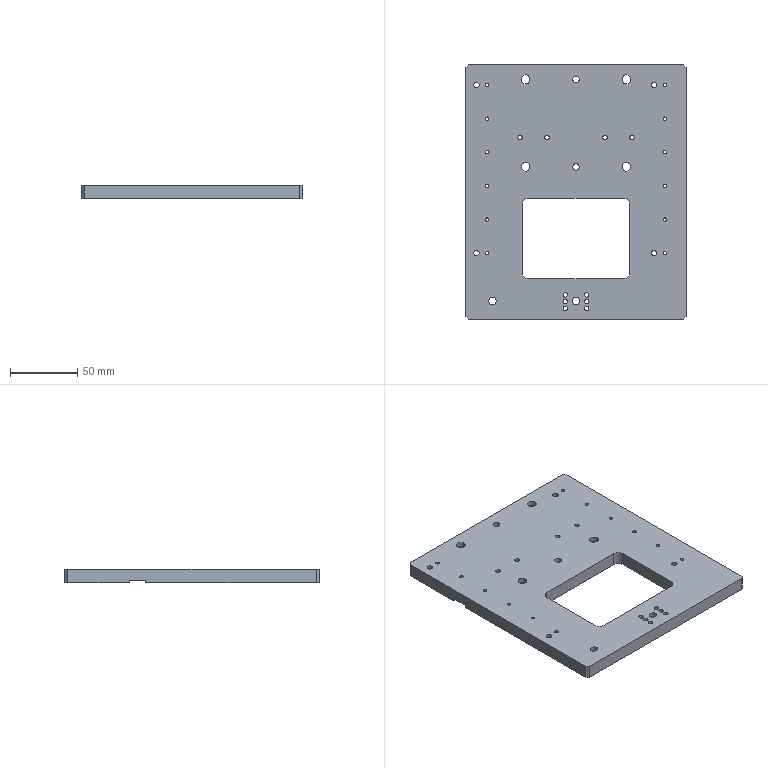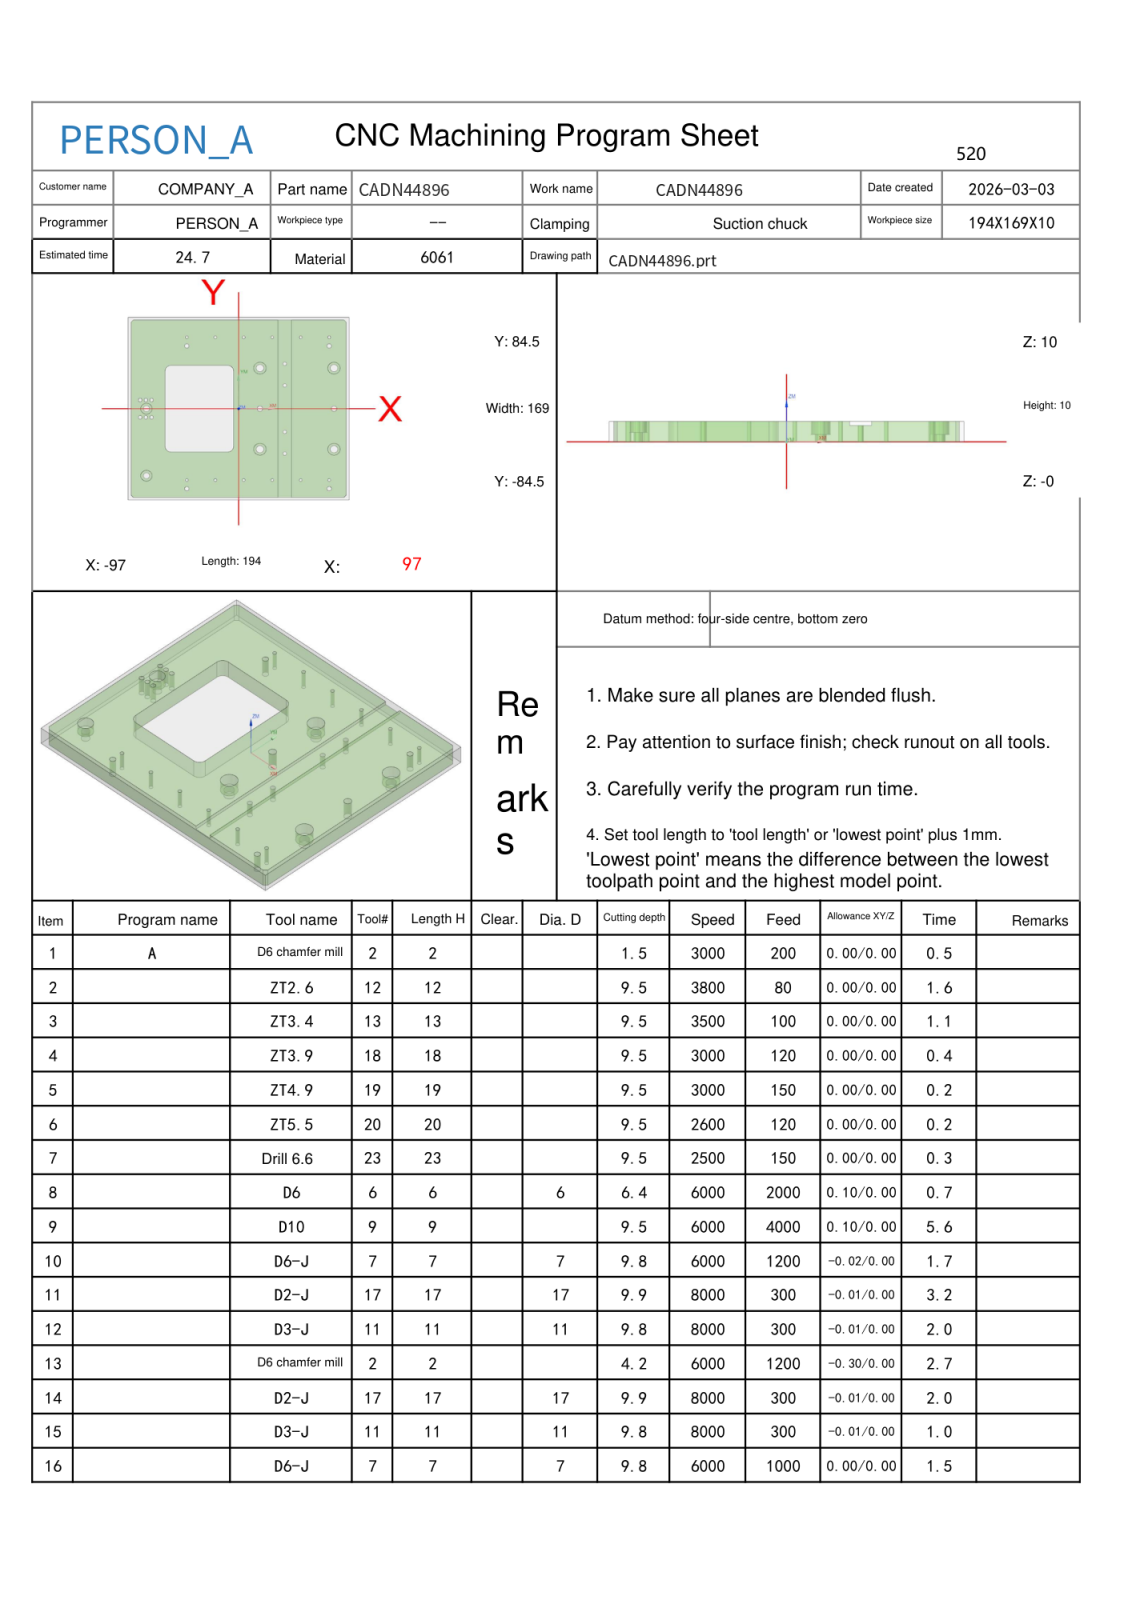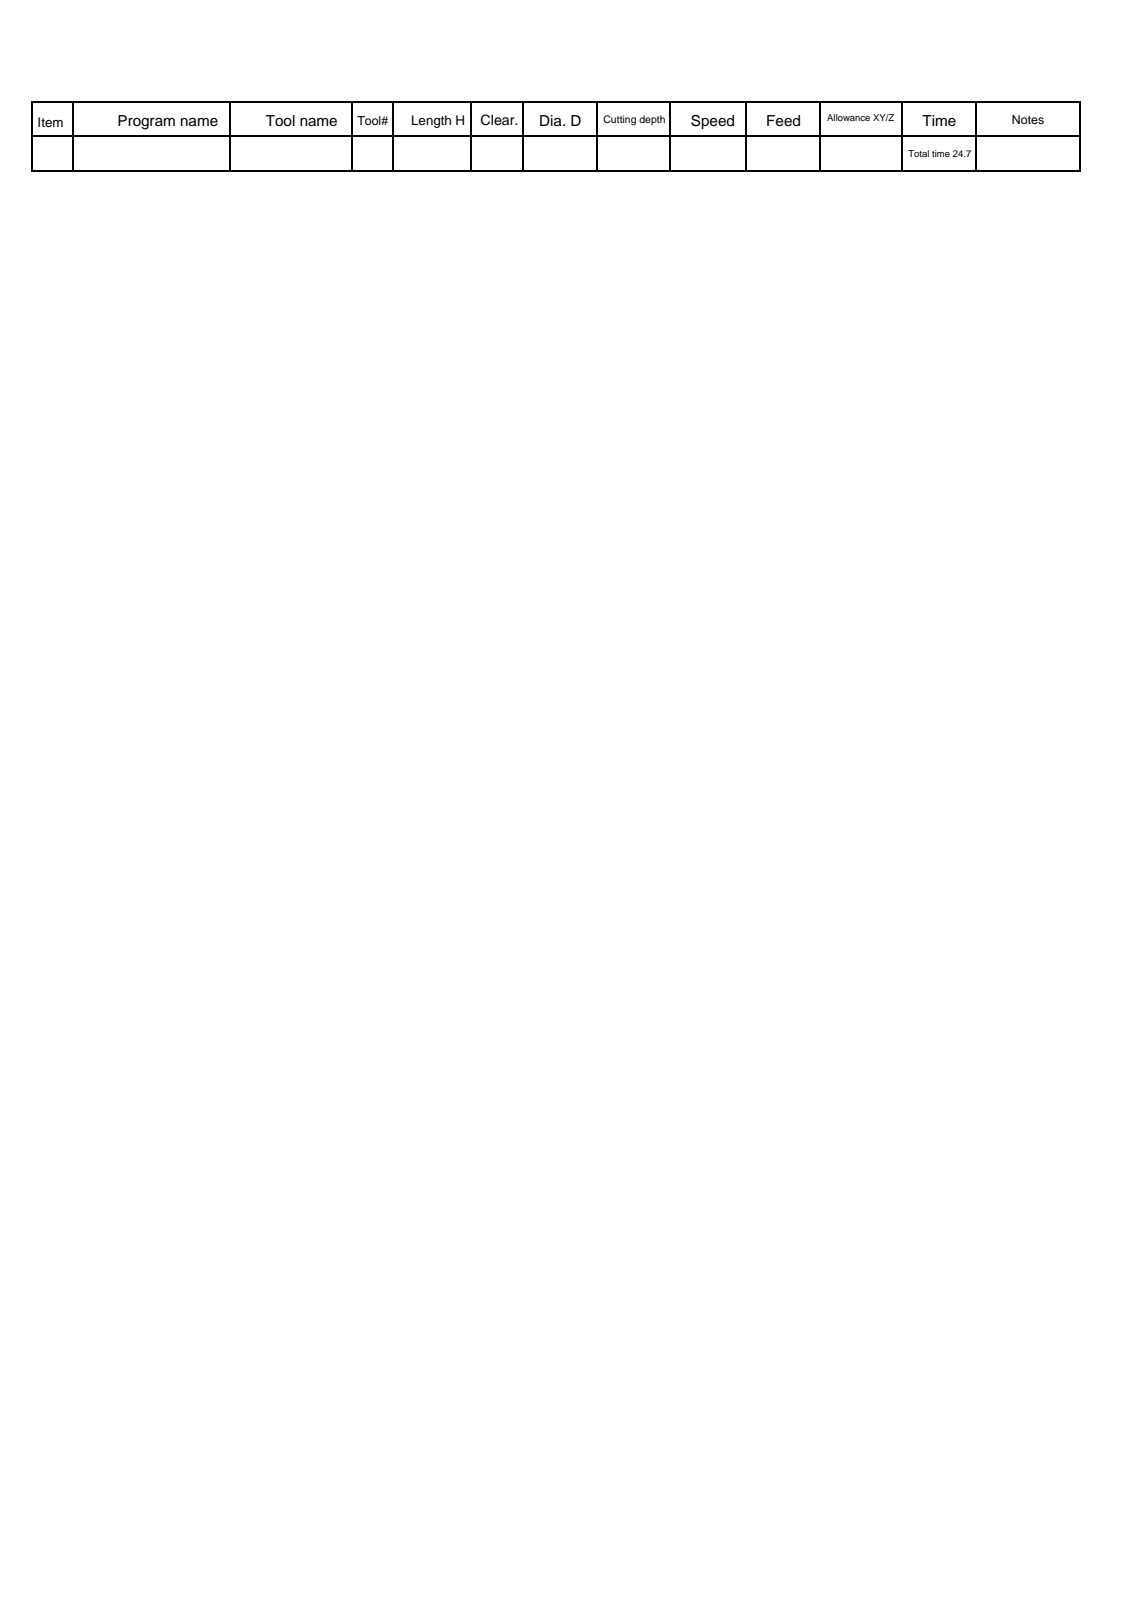NC program | NX | posted by the shop | part box 164 x 189 x 10 mm
Lines 1 to 1038 of 4061:
%
O0001
(Machine time: 27.66 MIN)
(===Total Tool:12===)
(T2=D6 chamfer mill   D=6.   R=0.   D-  H02 Z=5.8   )
(T12=ZT2.6  D=2.6  DR_a=118 D-  H12 Z=0.5   )
(T13=ZT3.4  D=3.4  DR_a=118 D-  H13 Z=0.5   )
(T18=ZT3.9  D=3.9  DR_a=120 D-  H18 Z=0.5   )
(T19=ZT4.9  D=4.9  DR_a=120 D-  H19 Z=0.5   )
(T20=ZT5.5  D=5.5  DR_a=118 D-  H20 Z=0.5   )
(T23=Drill 6.6  D=6.6  DR_a=120 D-  H23 Z=0.5   )
(T6=D6      D=6.   R=0.   D6  H06 Z=3.6   )
(T9=D10     D=10.  R=0.   D-  H09 Z=0.5   )
(T7=D6-J    D=6.   R=0.   D7  H07 Z=0.2   )
(T17=D2-J   D=2.   R=0.   D17 H17 Z=0.15  )
(T11=D3-J   D=3.   R=0.   D11 H11 Z=0.15  )
G80 G90 G17 G49 G40
G91 G28 Z0
M01
N1 T02 M06
(D6 chamfer mill  D=6. R=0. H=02 ce=0.00 di=0.00)
(MAX_Z=40. MIN_Z=8.5 Time=0.49M)
G00 G90 G54 X83.7 Y0.0 M03 S3000
G43 H02 Z40.
M08
G98 G82 X83.7 Y0.0 Z8.5 R11. F200.
X18.7
G80
G00 Z40.
G00 G90 X79.5 Y-66. M03 S3000
Z40.
G98 G81 X79.5 Y-66. Z9. R11. F200.
X54.5
X29.5
X4.5
X-20.5
X-45.5
Y66.
X-20.5
X4.5
X29.5
X54.5
X79.5
G80
G00 Z40.
G00 G90 X83.7 Y37.5 M03 S3000
Z40.
G98 G81 X83.7 Y37.5 Z8.5 R11. F200.
X79.5 Y58.
X40.5 Y41.5
X18.7 Y37.5
X40.5 Y21.5
Y-21.5
X83.7 Y-37.5
X79.5 Y-74.
X40.5 Y-41.5
X18.7 Y-37.5
X-45.5 Y-74.
X-81. Y-62.
X-86.5 Y-8.
X-81.5
X-76.5
X-81. Y0.0
X-86.5 Y8.
X-81.5
X-76.5
X-45.5 Y58.
G80
G00 Z40.
G91 G28 Z0.0
M05
M09
G91 G28 Z0.0
M01
N2 T12 M06
(ZT2.6 D=2.6 DR_a=118 H=12)
(MAX_Z=40. MIN_Z=0.5 Time=1.62M)
G00 G90 G54 X79.5 Y-66. M03 S3800
G43 H12 Z40.
M08
G98 G83 X79.5 Y-66. Z.5 R11. F80. Q1.5
X54.5
X29.5
X4.5
X-20.5
X-45.5
Y66.
X-20.5
X4.5
X29.5
X54.5
X79.5
G80
G00 Z40.
G91 G28 Z0.0
M05
M09
G91 G28 Z0.0
M01
N3 T13 M06
(ZT3.4 D=3.4 DR_a=118 H=13)
(MAX_Z=40. MIN_Z=0.5 Time=1.08M)
G00 G90 G54 X-76.5 Y-8. M03 S3500
G43 H13 Z40.
M08
G98 G83 X-76.5 Y-8. Z.5 R11. F100. Q1.5
X-81.5
X-86.5
Y8.
X-81.5
X-76.5
X40.5 Y41.5
Y21.5
Y-21.5
Y-41.5
G80
G00 Z40.
G91 G28 Z0.0
M05
M09
G91 G28 Z0.0
M01
N4 T18 M06
(ZT3.9 D=3.9 DR_a=120 H=18)
(MAX_Z=40. MIN_Z=0.5 Time=0.39M)
G00 G90 G54 X-45.5 Y-74. M03 S3000
G43 H18 Z40.
M08
G98 G83 X-45.5 Y-74. Z.5 R11. F120. Q2.
X79.5
Y58.
X-45.5
G80
G00 Z40.
G91 G28 Z0.0
M05
M09
G91 G28 Z0.0
M01
N5 T19 M06
(ZT4.9 D=4.9 DR_a=120 H=19)
(MAX_Z=40. MIN_Z=0.5 Time=0.16M)
G00 G90 G54 X83.7 Y0.0 M03 S3000
G43 H19 Z40.
M08
G98 G83 X83.7 Y0.0 Z.5 R11. F150. Q3.
X18.7
G80
G00 Z40.
G91 G28 Z0.0
M05
M09
G91 G28 Z0.0
M01
N6 T20 M06
(ZT5.5 D=5.5 DR_a=118 H=20)
(MAX_Z=40. MIN_Z=0.5 Time=0.19M)
G00 G90 G54 X-81. Y0.0 M03 S2600
G43 H20 Z40.
M08
G98 G83 X-81. Y0.0 Z.5 R11. F120. Q3.
Y-62.
G80
G00 Z40.
G91 G28 Z0.0
M05
M09
G91 G28 Z0.0
M01
N7 T23 M06
(Drill 6.6 D=6.6 DR_a=120 H=23)
(MAX_Z=40. MIN_Z=0.5 Time=0.31M)
G00 G90 G54 X83.7 Y37.5 M03 S2500
G43 H23 Z40.
M08
G98 G83 X83.7 Y37.5 Z.5 R11. F150. Q3.
X18.7
Y-37.5
X83.7
G80
G00 Z40.
G91 G28 Z0.0
M05
M09
G91 G28 Z0.0
M01
N8 T06 M06
(D6  D=6. R=0. H=06 ce=0.10 di=0.00)
(D.N=06 MAX_Z=40. MIN_Z=3.6 Time=0.72M)
G00 G90 G54 X-81. Y0.0 M03 S6000
G43 H06 Z40.
M08
Z10.3
G41 D06
G01 X-80.9 Y-.007 F2000.
G03 X-80.044 Y.944 I-.1 J.951
X-81. Y1.9 I-.956 J0.0
X-81. Y1.9 Z9.95 I0.0 J-1.9
X-81. Y1.9 Z9.6 I0.0 J-1.9
X-81. Y1.9 Z9.25 I0.0 J-1.9
X-81. Y1.9 Z8.9 I0.0 J-1.9
X-81. Y1.9 Z8.55 I0.0 J-1.9
X-81. Y1.9 Z8.2 I0.0 J-1.9
X-81. Y1.9 Z7.85 I0.0 J-1.9
X-81. Y1.9 Z7.5 I0.0 J-1.9
X-81. Y1.9 Z7.15 I0.0 J-1.9
X-81. Y1.9 Z6.8 I0.0 J-1.9
X-81. Y1.9 Z6.45 I0.0 J-1.9
X-81. Y1.9 Z6.1 I0.0 J-1.9
X-81. Y1.9 Z5.75 I0.0 J-1.9
X-81. Y1.9 Z5.4 I0.0 J-1.9
X-81. Y1.9 Z5.05 I0.0 J-1.9
X-81. Y1.9 Z4.7 I0.0 J-1.9
X-82.852 Y-.423 Z4.6 I0.0 J-1.9
X-81. Y-1.9 I1.852 J.423
X-79.1 Y0.0 I0.0 J1.9
X-81. Y1.9 I-1.9 J0.0
X-82.9 Y0.0 I0.0 J-1.9
X-82.852 Y-.423 I1.9 J0.0
X-81.92 Y-1.166 I.932 J.213
X-80.964 Y-.21 I0.0 J.956
G01 X-80.971 Y-.096
G40 X-81. Y0.0
G00 Z40.
Y-62.
Z10.3
G41 D06
G01 X-80.9 Y-62.007
G03 X-80.044 Y-61.056 I-.1 J.951
X-81. Y-60.1 I-.956 J0.0
X-81. Y-60.1 Z9.95 I0.0 J-1.9
X-81. Y-60.1 Z9.6 I0.0 J-1.9
X-81. Y-60.1 Z9.25 I0.0 J-1.9
X-81. Y-60.1 Z8.9 I0.0 J-1.9
X-81. Y-60.1 Z8.55 I0.0 J-1.9
X-81. Y-60.1 Z8.2 I0.0 J-1.9
X-81. Y-60.1 Z7.85 I0.0 J-1.9
X-81. Y-60.1 Z7.5 I0.0 J-1.9
X-81. Y-60.1 Z7.15 I0.0 J-1.9
X-81. Y-60.1 Z6.8 I0.0 J-1.9
X-81. Y-60.1 Z6.45 I0.0 J-1.9
X-81. Y-60.1 Z6.1 I0.0 J-1.9
X-81. Y-60.1 Z5.75 I0.0 J-1.9
X-81. Y-60.1 Z5.4 I0.0 J-1.9
X-81. Y-60.1 Z5.05 I0.0 J-1.9
X-81. Y-60.1 Z4.7 I0.0 J-1.9
X-82.852 Y-62.423 Z4.6 I0.0 J-1.9
X-81. Y-63.9 I1.852 J.423
X-79.1 Y-62. I0.0 J1.9
X-81. Y-60.1 I-1.9 J0.0
X-82.9 Y-62. I0.0 J-1.9
X-82.852 Y-62.423 I1.9 J0.0
X-81.92 Y-63.166 I.932 J.213
X-80.964 Y-62.21 I0.0 J.956
G01 X-80.971 Y-62.096
G40 X-81. Y-62.
G00 Z40.
G00 G90 X18.7 Y-37.5 M03 S6000
Z40.
Z10.3
G03 X19.9 Y-36.3 I0.0 J1.2 F2000.
X18.7 Y-35.1 I-1.2 J0.0
X18.7 Y-35.1 Z9.8 I0.0 J-2.4
X18.7 Y-35.1 Z9.3 I0.0 J-2.4
X18.7 Y-35.1 Z8.8 I0.0 J-2.4
X18.7 Y-35.1 Z8.3 I0.0 J-2.4
X18.7 Y-35.1 Z7.8 I0.0 J-2.4
X18.7 Y-35.1 Z7.3 I0.0 J-2.4
X18.7 Y-35.1 Z6.8 I0.0 J-2.4
X18.7 Y-35.1 Z6.3 I0.0 J-2.4
X18.7 Y-35.1 Z5.8 I0.0 J-2.4
X18.7 Y-35.1 Z5.3 I0.0 J-2.4
X18.7 Y-35.1 Z4.8 I0.0 J-2.4
X18.7 Y-35.1 Z4.3 I0.0 J-2.4
X18.7 Y-35.1 Z3.8 I0.0 J-2.4
X17.289 Y-39.442 Z3.6 I0.0 J-2.4
X18.7 Y-39.9 I1.411 J1.942
X21.1 Y-37.5 I0.0 J2.4
X18.7 Y-35.1 I-2.4 J0.0
X16.3 Y-37.5 I0.0 J-2.4
X17.289 Y-39.442 I2.4 J0.0
X17.995 Y-39.671 I.705 J.971
X19.195 Y-38.471 I0.0 J1.2
X18.7 Y-37.5 I-1.2 J0.0
G00 Z40.
X83.7
Z10.3
G03 X84.9 Y-36.3 I0.0 J1.2
X83.7 Y-35.1 I-1.2 J0.0
X83.7 Y-35.1 Z9.8 I0.0 J-2.4
X83.7 Y-35.1 Z9.3 I0.0 J-2.4
X83.7 Y-35.1 Z8.8 I0.0 J-2.4
X83.7 Y-35.1 Z8.3 I0.0 J-2.4
X83.7 Y-35.1 Z7.8 I0.0 J-2.4
X83.7 Y-35.1 Z7.3 I0.0 J-2.4
X83.7 Y-35.1 Z6.8 I0.0 J-2.4
X83.7 Y-35.1 Z6.3 I0.0 J-2.4
X83.7 Y-35.1 Z5.8 I0.0 J-2.4
X83.7 Y-35.1 Z5.3 I0.0 J-2.4
X83.7 Y-35.1 Z4.8 I0.0 J-2.4
X83.7 Y-35.1 Z4.3 I0.0 J-2.4
X83.7 Y-35.1 Z3.8 I0.0 J-2.4
X82.289 Y-39.442 Z3.6 I0.0 J-2.4
X83.7 Y-39.9 I1.411 J1.942
X86.1 Y-37.5 I0.0 J2.4
X83.7 Y-35.1 I-2.4 J0.0
X81.3 Y-37.5 I0.0 J-2.4
X82.289 Y-39.442 I2.4 J0.0
X82.995 Y-39.671 I.705 J.971
X84.195 Y-38.471 I0.0 J1.2
X83.7 Y-37.5 I-1.2 J0.0
G00 Z40.
Y37.5
Z10.3
G03 X84.9 Y38.7 I0.0 J1.2
X83.7 Y39.9 I-1.2 J0.0
X83.7 Y39.9 Z9.8 I0.0 J-2.4
X83.7 Y39.9 Z9.3 I0.0 J-2.4
X83.7 Y39.9 Z8.8 I0.0 J-2.4
X83.7 Y39.9 Z8.3 I0.0 J-2.4
X83.7 Y39.9 Z7.8 I0.0 J-2.4
X83.7 Y39.9 Z7.3 I0.0 J-2.4
X83.7 Y39.9 Z6.8 I0.0 J-2.4
X83.7 Y39.9 Z6.3 I0.0 J-2.4
X83.7 Y39.9 Z5.8 I0.0 J-2.4
X83.7 Y39.9 Z5.3 I0.0 J-2.4
X83.7 Y39.9 Z4.8 I0.0 J-2.4
X83.7 Y39.9 Z4.3 I0.0 J-2.4
X83.7 Y39.9 Z3.8 I0.0 J-2.4
X82.289 Y35.558 Z3.6 I0.0 J-2.4
X83.7 Y35.1 I1.411 J1.942
X86.1 Y37.5 I0.0 J2.4
X83.7 Y39.9 I-2.4 J0.0
X81.3 Y37.5 I0.0 J-2.4
X82.289 Y35.558 I2.4 J0.0
X82.995 Y35.329 I.705 J.971
X84.195 Y36.529 I0.0 J1.2
X83.7 Y37.5 I-1.2 J0.0
G00 Z40.
X18.7
Z10.3
G03 X19.9 Y38.7 I0.0 J1.2
X18.7 Y39.9 I-1.2 J0.0
X18.7 Y39.9 Z9.8 I0.0 J-2.4
X18.7 Y39.9 Z9.3 I0.0 J-2.4
X18.7 Y39.9 Z8.8 I0.0 J-2.4
X18.7 Y39.9 Z8.3 I0.0 J-2.4
X18.7 Y39.9 Z7.8 I0.0 J-2.4
X18.7 Y39.9 Z7.3 I0.0 J-2.4
X18.7 Y39.9 Z6.8 I0.0 J-2.4
X18.7 Y39.9 Z6.3 I0.0 J-2.4
X18.7 Y39.9 Z5.8 I0.0 J-2.4
X18.7 Y39.9 Z5.3 I0.0 J-2.4
X18.7 Y39.9 Z4.8 I0.0 J-2.4
X18.7 Y39.9 Z4.3 I0.0 J-2.4
X18.7 Y39.9 Z3.8 I0.0 J-2.4
X17.289 Y35.558 Z3.6 I0.0 J-2.4
X18.7 Y35.1 I1.411 J1.942
X21.1 Y37.5 I0.0 J2.4
X18.7 Y39.9 I-2.4 J0.0
X16.3 Y37.5 I0.0 J-2.4
X17.289 Y35.558 I2.4 J0.0
X17.995 Y35.329 I.705 J.971
X19.195 Y36.529 I0.0 J1.2
X18.7 Y37.5 I-1.2 J0.0
G00 Z40.
G91 G28 Z0.0
M05
M09
G91 G28 Z0.0
M01
N9 T09 M06
(D10  D=10. R=0. H=09 ce=0.10 di=0.10)
(MAX_Z=40. MIN_Z=0.5 Time=5.57M)
G00 G90 G54 X41.4 Y46.666 M03 S6000
G43 H09 Z40.
M08
Z10.5
G01 Y83. Z9.549 F3500.
X40.5 Z9.525
X39.6
Y-83.
X41.4
Y83.
X40.5
X40.
Z10.025
G00 Z10.5
X41.4 Y46.666
Z10.025
G01 Y83. Z9.074
X40.5 Z9.05
X39.6
Y-83.
X41.4
Y83.
X40.5
X40.
Z9.55
G00 Z10.025
X41.4 Y46.666
Z9.55
G01 Y83. Z8.599
X40.5 Z8.575
X39.6
Y-83.
X41.4
Y83.
X40.5
X40.
Z9.075
G00 Z9.55
X41.4 Y46.666
Z9.075
G01 Y83. Z8.124
X40.5 Z8.1
X39.6
Y-83.
X41.4
Y83.
X40.5
X40.
Z8.6
G00 Z40.
G00 G90 X-59.4 Y0.0 M03 S6000
Z40.
Z10.5
G01 Y-34.9 Z10.427 F4000.
X-9.6 Z10.323
Y34.9 Z10.177
X-59.4 Z10.073
Y-34.9 Z9.927
X-9.6 Z9.823
Y34.9 Z9.677
X-59.4 Z9.573
Y-34.9 Z9.427
X-9.6 Z9.323
Y34.9 Z9.177
X-59.4 Z9.073
Y-34.9 Z8.927
X-9.6 Z8.823
Y34.9 Z8.677
X-59.4 Z8.573
Y-34.9 Z8.427
X-9.6 Z8.323
Y34.9 Z8.177
X-59.4 Z8.073
Y-34.9 Z7.927
X-9.6 Z7.823
Y34.9 Z7.677
X-59.4 Z7.573
Y-34.9 Z7.427
X-9.6 Z7.323
Y34.9 Z7.177
X-59.4 Z7.073
Y-34.9 Z6.927
X-9.6 Z6.823
Y34.9 Z6.677
X-59.4 Z6.573
Y-34.9 Z6.427
X-9.6 Z6.323
Y34.9 Z6.177
X-59.4 Z6.073
Y-34.9 Z5.927
X-9.6 Z5.823
Y34.9 Z5.677
X-59.4 Z5.573
Y-34.9 Z5.427
X-9.6 Z5.323
Y34.9 Z5.177
X-59.4 Z5.073
Y-34.9 Z4.927
X-9.6 Z4.823
Y34.9 Z4.677
X-59.4 Z4.573
Y-34.9 Z4.427
X-9.6 Z4.323
Y34.9 Z4.177
X-59.4 Z4.073
Y-34.9 Z3.927
X-9.6 Z3.823
Y34.9 Z3.677
X-59.4 Z3.573
Y-34.9 Z3.427
X-9.6 Z3.323
Y34.9 Z3.177
X-59.4 Z3.073
Y-34.9 Z2.927
X-9.6 Z2.823
Y34.9 Z2.677
X-59.4 Z2.573
Y-34.9 Z2.427
X-9.6 Z2.323
Y34.9 Z2.177
X-59.4 Z2.073
Y-34.9 Z1.927
X-9.6 Z1.823
Y34.9 Z1.677
X-59.4 Z1.573
Y-34.9 Z1.427
X-9.6 Z1.323
Y34.9 Z1.177
X-59.4 Z1.073
Y-34.9 Z.927
X-9.6 Z.823
Y34.9 Z.677
X-59.4 Z.573
Y0.0 Z.5
Y-34.9
X-9.6
Y34.9
X-59.4
Y0.0
Y-.5
Z1.5
G00 Z40.
G00 G90 X0.0 Y-87.1 M03 S6000
Z40.
Z10.5
G01 X-92.5 Z10.437 F4000.
G02 X-96.106 Y-85.606 Z10.434 I0.0 J5.1
G01 X-98.106 Y-83.606 Z10.432
G02 X-99.6 Y-80. Z10.43 I3.606 J3.606
G01 Y80. Z10.32
G02 X-98.106 Y83.606 Z10.318 I5.1 J0.0
G01 X-96.106 Y85.606 Z10.316
G02 X-92.5 Y87.1 Z10.313 I3.606 J-3.606
G01 X92.5 Z10.187
G02 X96.106 Y85.606 Z10.184 I0.0 J-5.1
G01 X98.106 Y83.606 Z10.182
G02 X99.6 Y80. Z10.18 I-3.606 J-3.606
G01 Y-80. Z10.07
G02 X98.106 Y-83.606 Z10.068 I-5.1 J0.0
G01 X96.106 Y-85.606 Z10.066
G02 X92.5 Y-87.1 Z10.063 I-3.606 J3.606
G01 X-92.5 Z9.937
G02 X-96.106 Y-85.606 Z9.934 I0.0 J5.1
G01 X-98.106 Y-83.606 Z9.932
G02 X-99.6 Y-80. Z9.93 I3.606 J3.606
G01 Y80. Z9.82
G02 X-98.106 Y83.606 Z9.818 I5.1 J0.0
G01 X-96.106 Y85.606 Z9.816
G02 X-92.5 Y87.1 Z9.813 I3.606 J-3.606
G01 X92.5 Z9.687
G02 X96.106 Y85.606 Z9.684 I0.0 J-5.1
G01 X98.106 Y83.606 Z9.682
G02 X99.6 Y80. Z9.68 I-3.606 J-3.606
G01 Y-80. Z9.57
G02 X98.106 Y-83.606 Z9.568 I-5.1 J0.0
G01 X96.106 Y-85.606 Z9.566
G02 X92.5 Y-87.1 Z9.563 I-3.606 J3.606
G01 X-92.5 Z9.437
G02 X-96.106 Y-85.606 Z9.434 I0.0 J5.1
G01 X-98.106 Y-83.606 Z9.432
G02 X-99.6 Y-80. Z9.43 I3.606 J3.606
G01 Y80. Z9.32
G02 X-98.106 Y83.606 Z9.318 I5.1 J0.0
G01 X-96.106 Y85.606 Z9.316
G02 X-92.5 Y87.1 Z9.313 I3.606 J-3.606
G01 X92.5 Z9.187
G02 X96.106 Y85.606 Z9.184 I0.0 J-5.1
G01 X98.106 Y83.606 Z9.182
G02 X99.6 Y80. Z9.18 I-3.606 J-3.606
G01 Y-80. Z9.07
G02 X98.106 Y-83.606 Z9.068 I-5.1 J0.0
G01 X96.106 Y-85.606 Z9.066
G02 X92.5 Y-87.1 Z9.063 I-3.606 J3.606
G01 X-92.5 Z8.937
G02 X-96.106 Y-85.606 Z8.934 I0.0 J5.1
G01 X-98.106 Y-83.606 Z8.932
G02 X-99.6 Y-80. Z8.93 I3.606 J3.606
G01 Y80. Z8.82
G02 X-98.106 Y83.606 Z8.818 I5.1 J0.0
G01 X-96.106 Y85.606 Z8.816
G02 X-92.5 Y87.1 Z8.813 I3.606 J-3.606
G01 X92.5 Z8.687
G02 X96.106 Y85.606 Z8.684 I0.0 J-5.1
G01 X98.106 Y83.606 Z8.682
G02 X99.6 Y80. Z8.68 I-3.606 J-3.606
G01 Y-80. Z8.57
G02 X98.106 Y-83.606 Z8.568 I-5.1 J0.0
G01 X96.106 Y-85.606 Z8.566
G02 X92.5 Y-87.1 Z8.563 I-3.606 J3.606
G01 X-92.5 Z8.437
G02 X-96.106 Y-85.606 Z8.434 I0.0 J5.1
G01 X-98.106 Y-83.606 Z8.432
G02 X-99.6 Y-80. Z8.43 I3.606 J3.606
G01 Y80. Z8.32
G02 X-98.106 Y83.606 Z8.318 I5.1 J0.0
G01 X-96.106 Y85.606 Z8.316
G02 X-92.5 Y87.1 Z8.313 I3.606 J-3.606
G01 X92.5 Z8.187
G02 X96.106 Y85.606 Z8.184 I0.0 J-5.1
G01 X98.106 Y83.606 Z8.182
G02 X99.6 Y80. Z8.18 I-3.606 J-3.606
G01 Y-80. Z8.07
G02 X98.106 Y-83.606 Z8.068 I-5.1 J0.0
G01 X96.106 Y-85.606 Z8.066
G02 X92.5 Y-87.1 Z8.063 I-3.606 J3.606
G01 X-92.5 Z7.937
G02 X-96.106 Y-85.606 Z7.934 I0.0 J5.1
G01 X-98.106 Y-83.606 Z7.932
G02 X-99.6 Y-80. Z7.93 I3.606 J3.606
G01 Y80. Z7.82
G02 X-98.106 Y83.606 Z7.818 I5.1 J0.0
G01 X-96.106 Y85.606 Z7.816
G02 X-92.5 Y87.1 Z7.813 I3.606 J-3.606
G01 X92.5 Z7.687
G02 X96.106 Y85.606 Z7.684 I0.0 J-5.1
G01 X98.106 Y83.606 Z7.682
G02 X99.6 Y80. Z7.68 I-3.606 J-3.606
G01 Y-80. Z7.57
G02 X98.106 Y-83.606 Z7.568 I-5.1 J0.0
G01 X96.106 Y-85.606 Z7.566
G02 X92.5 Y-87.1 Z7.563 I-3.606 J3.606
G01 X-92.5 Z7.437
G02 X-96.106 Y-85.606 Z7.434 I0.0 J5.1
G01 X-98.106 Y-83.606 Z7.432
G02 X-99.6 Y-80. Z7.43 I3.606 J3.606
G01 Y80. Z7.32
G02 X-98.106 Y83.606 Z7.318 I5.1 J0.0
G01 X-96.106 Y85.606 Z7.316
G02 X-92.5 Y87.1 Z7.313 I3.606 J-3.606
G01 X92.5 Z7.187
G02 X96.106 Y85.606 Z7.184 I0.0 J-5.1
G01 X98.106 Y83.606 Z7.182
G02 X99.6 Y80. Z7.18 I-3.606 J-3.606
G01 Y-80. Z7.07
G02 X98.106 Y-83.606 Z7.068 I-5.1 J0.0
G01 X96.106 Y-85.606 Z7.066
G02 X92.5 Y-87.1 Z7.063 I-3.606 J3.606
G01 X-92.5 Z6.937
G02 X-96.106 Y-85.606 Z6.934 I0.0 J5.1
G01 X-98.106 Y-83.606 Z6.932
G02 X-99.6 Y-80. Z6.93 I3.606 J3.606
G01 Y80. Z6.82
G02 X-98.106 Y83.606 Z6.818 I5.1 J0.0
G01 X-96.106 Y85.606 Z6.816
G02 X-92.5 Y87.1 Z6.813 I3.606 J-3.606
G01 X92.5 Z6.687
G02 X96.106 Y85.606 Z6.684 I0.0 J-5.1
G01 X98.106 Y83.606 Z6.682
G02 X99.6 Y80. Z6.68 I-3.606 J-3.606
G01 Y-80. Z6.57
G02 X98.106 Y-83.606 Z6.568 I-5.1 J0.0
G01 X96.106 Y-85.606 Z6.566
G02 X92.5 Y-87.1 Z6.563 I-3.606 J3.606
G01 X-92.5 Z6.437
G02 X-96.106 Y-85.606 Z6.434 I0.0 J5.1
G01 X-98.106 Y-83.606 Z6.432
G02 X-99.6 Y-80. Z6.43 I3.606 J3.606
G01 Y80. Z6.32
G02 X-98.106 Y83.606 Z6.318 I5.1 J0.0
G01 X-96.106 Y85.606 Z6.316
G02 X-92.5 Y87.1 Z6.313 I3.606 J-3.606
G01 X92.5 Z6.187
G02 X96.106 Y85.606 Z6.184 I0.0 J-5.1
G01 X98.106 Y83.606 Z6.182
G02 X99.6 Y80. Z6.18 I-3.606 J-3.606
G01 Y-80. Z6.07
G02 X98.106 Y-83.606 Z6.068 I-5.1 J0.0
G01 X96.106 Y-85.606 Z6.066
G02 X92.5 Y-87.1 Z6.063 I-3.606 J3.606
G01 X-92.5 Z5.937
G02 X-96.106 Y-85.606 Z5.934 I0.0 J5.1
G01 X-98.106 Y-83.606 Z5.932
G02 X-99.6 Y-80. Z5.93 I3.606 J3.606
G01 Y80. Z5.82
G02 X-98.106 Y83.606 Z5.818 I5.1 J0.0
G01 X-96.106 Y85.606 Z5.816
G02 X-92.5 Y87.1 Z5.813 I3.606 J-3.606
G01 X92.5 Z5.687
G02 X96.106 Y85.606 Z5.684 I0.0 J-5.1
G01 X98.106 Y83.606 Z5.682
G02 X99.6 Y80. Z5.68 I-3.606 J-3.606
G01 Y-80. Z5.57
G02 X98.106 Y-83.606 Z5.568 I-5.1 J0.0
G01 X96.106 Y-85.606 Z5.566
G02 X92.5 Y-87.1 Z5.563 I-3.606 J3.606
G01 X-92.5 Z5.437
G02 X-96.106 Y-85.606 Z5.434 I0.0 J5.1
G01 X-98.106 Y-83.606 Z5.432
G02 X-99.6 Y-80. Z5.43 I3.606 J3.606
G01 Y80. Z5.32
G02 X-98.106 Y83.606 Z5.318 I5.1 J0.0
G01 X-96.106 Y85.606 Z5.316
G02 X-92.5 Y87.1 Z5.313 I3.606 J-3.606
G01 X92.5 Z5.187
G02 X96.106 Y85.606 Z5.184 I0.0 J-5.1
G01 X98.106 Y83.606 Z5.182
G02 X99.6 Y80. Z5.18 I-3.606 J-3.606
G01 Y-80. Z5.07
G02 X98.106 Y-83.606 Z5.068 I-5.1 J0.0
G01 X96.106 Y-85.606 Z5.066
G02 X92.5 Y-87.1 Z5.063 I-3.606 J3.606
G01 X-92.5 Z4.937
G02 X-96.106 Y-85.606 Z4.934 I0.0 J5.1
G01 X-98.106 Y-83.606 Z4.932
G02 X-99.6 Y-80. Z4.93 I3.606 J3.606
G01 Y80. Z4.82
G02 X-98.106 Y83.606 Z4.818 I5.1 J0.0
G01 X-96.106 Y85.606 Z4.816
G02 X-92.5 Y87.1 Z4.813 I3.606 J-3.606
G01 X92.5 Z4.687
G02 X96.106 Y85.606 Z4.684 I0.0 J-5.1
G01 X98.106 Y83.606 Z4.682
G02 X99.6 Y80. Z4.68 I-3.606 J-3.606
G01 Y-80. Z4.57
G02 X98.106 Y-83.606 Z4.568 I-5.1 J0.0
G01 X96.106 Y-85.606 Z4.566
G02 X92.5 Y-87.1 Z4.563 I-3.606 J3.606
G01 X-92.5 Z4.437
G02 X-96.106 Y-85.606 Z4.434 I0.0 J5.1
G01 X-98.106 Y-83.606 Z4.432
G02 X-99.6 Y-80. Z4.43 I3.606 J3.606
G01 Y80. Z4.32
G02 X-98.106 Y83.606 Z4.318 I5.1 J0.0
G01 X-96.106 Y85.606 Z4.316
G02 X-92.5 Y87.1 Z4.313 I3.606 J-3.606
G01 X92.5 Z4.187
G02 X96.106 Y85.606 Z4.184 I0.0 J-5.1
G01 X98.106 Y83.606 Z4.182
G02 X99.6 Y80. Z4.18 I-3.606 J-3.606
G01 Y-80. Z4.07
G02 X98.106 Y-83.606 Z4.068 I-5.1 J0.0
G01 X96.106 Y-85.606 Z4.066
G02 X92.5 Y-87.1 Z4.063 I-3.606 J3.606
G01 X-92.5 Z3.937
G02 X-96.106 Y-85.606 Z3.934 I0.0 J5.1
G01 X-98.106 Y-83.606 Z3.932
G02 X-99.6 Y-80. Z3.93 I3.606 J3.606
G01 Y80. Z3.82
G02 X-98.106 Y83.606 Z3.818 I5.1 J0.0
G01 X-96.106 Y85.606 Z3.816
G02 X-92.5 Y87.1 Z3.813 I3.606 J-3.606
G01 X92.5 Z3.687
G02 X96.106 Y85.606 Z3.684 I0.0 J-5.1
G01 X98.106 Y83.606 Z3.682
G02 X99.6 Y80. Z3.68 I-3.606 J-3.606
G01 Y-80. Z3.57
G02 X98.106 Y-83.606 Z3.568 I-5.1 J0.0
G01 X96.106 Y-85.606 Z3.566
G02 X92.5 Y-87.1 Z3.563 I-3.606 J3.606
G01 X-92.5 Z3.437
G02 X-96.106 Y-85.606 Z3.434 I0.0 J5.1
G01 X-98.106 Y-83.606 Z3.432
G02 X-99.6 Y-80. Z3.43 I3.606 J3.606
G01 Y80. Z3.32
G02 X-98.106 Y83.606 Z3.318 I5.1 J0.0
G01 X-96.106 Y85.606 Z3.316
G02 X-92.5 Y87.1 Z3.313 I3.606 J-3.606
G01 X92.5 Z3.187
G02 X96.106 Y85.606 Z3.184 I0.0 J-5.1
G01 X98.106 Y83.606 Z3.182
G02 X99.6 Y80. Z3.18 I-3.606 J-3.606
G01 Y-80. Z3.07
G02 X98.106 Y-83.606 Z3.068 I-5.1 J0.0
G01 X96.106 Y-85.606 Z3.066
G02 X92.5 Y-87.1 Z3.063 I-3.606 J3.606
G01 X-92.5 Z2.937
G02 X-96.106 Y-85.606 Z2.934 I0.0 J5.1
G01 X-98.106 Y-83.606 Z2.932
G02 X-99.6 Y-80. Z2.93 I3.606 J3.606
G01 Y80. Z2.82
G02 X-98.106 Y83.606 Z2.818 I5.1 J0.0
G01 X-96.106 Y85.606 Z2.816
G02 X-92.5 Y87.1 Z2.813 I3.606 J-3.606
G01 X92.5 Z2.687
G02 X96.106 Y85.606 Z2.684 I0.0 J-5.1
G01 X98.106 Y83.606 Z2.682
G02 X99.6 Y80. Z2.68 I-3.606 J-3.606
G01 Y-80. Z2.57
G02 X98.106 Y-83.606 Z2.568 I-5.1 J0.0
G01 X96.106 Y-85.606 Z2.566
G02 X92.5 Y-87.1 Z2.563 I-3.606 J3.606
G01 X-92.5 Z2.437
G02 X-96.106 Y-85.606 Z2.434 I0.0 J5.1
G01 X-98.106 Y-83.606 Z2.432
G02 X-99.6 Y-80. Z2.43 I3.606 J3.606
G01 Y80. Z2.32
G02 X-98.106 Y83.606 Z2.318 I5.1 J0.0
G01 X-96.106 Y85.606 Z2.316
G02 X-92.5 Y87.1 Z2.313 I3.606 J-3.606
G01 X92.5 Z2.187
G02 X96.106 Y85.606 Z2.184 I0.0 J-5.1
G01 X98.106 Y83.606 Z2.182
G02 X99.6 Y80. Z2.18 I-3.606 J-3.606
G01 Y-80. Z2.07
G02 X98.106 Y-83.606 Z2.068 I-5.1 J0.0
G01 X96.106 Y-85.606 Z2.066
G02 X92.5 Y-87.1 Z2.063 I-3.606 J3.606
G01 X-92.5 Z1.937
G02 X-96.106 Y-85.606 Z1.934 I0.0 J5.1
G01 X-98.106 Y-83.606 Z1.932
G02 X-99.6 Y-80. Z1.93 I3.606 J3.606
G01 Y80. Z1.82
G02 X-98.106 Y83.606 Z1.818 I5.1 J0.0
G01 X-96.106 Y85.606 Z1.816
G02 X-92.5 Y87.1 Z1.813 I3.606 J-3.606
G01 X92.5 Z1.687
G02 X96.106 Y85.606 Z1.684 I0.0 J-5.1
G01 X98.106 Y83.606 Z1.682
G02 X99.6 Y80. Z1.68 I-3.606 J-3.606
G01 Y-80. Z1.57
G02 X98.106 Y-83.606 Z1.568 I-5.1 J0.0
G01 X96.106 Y-85.606 Z1.566
G02 X92.5 Y-87.1 Z1.563 I-3.606 J3.606
G01 X-92.5 Z1.437
G02 X-96.106 Y-85.606 Z1.434 I0.0 J5.1
G01 X-98.106 Y-83.606 Z1.432
G02 X-99.6 Y-80. Z1.43 I3.606 J3.606
G01 Y80. Z1.32
G02 X-98.106 Y83.606 Z1.318 I5.1 J0.0
G01 X-96.106 Y85.606 Z1.316
G02 X-92.5 Y87.1 Z1.313 I3.606 J-3.606
G01 X92.5 Z1.187
G02 X96.106 Y85.606 Z1.184 I0.0 J-5.1
G01 X98.106 Y83.606 Z1.182
G02 X99.6 Y80. Z1.18 I-3.606 J-3.606
G01 Y-80. Z1.07
G02 X98.106 Y-83.606 Z1.068 I-5.1 J0.0
G01 X96.106 Y-85.606 Z1.066
G02 X92.5 Y-87.1 Z1.063 I-3.606 J3.606
G01 X-92.5 Z.937
G02 X-96.106 Y-85.606 Z.934 I0.0 J5.1
G01 X-98.106 Y-83.606 Z.932
G02 X-99.6 Y-80. Z.93 I3.606 J3.606
G01 Y80. Z.82
G02 X-98.106 Y83.606 Z.818 I5.1 J0.0
G01 X-96.106 Y85.606 Z.816
G02 X-92.5 Y87.1 Z.813 I3.606 J-3.606
G01 X92.5 Z.687
G02 X96.106 Y85.606 Z.684 I0.0 J-5.1
G01 X98.106 Y83.606 Z.682
G02 X99.6 Y80. Z.68 I-3.606 J-3.606
G01 Y-80. Z.57
G02 X98.106 Y-83.606 Z.568 I-5.1 J0.0
G01 X96.106 Y-85.606 Z.566
G02 X92.5 Y-87.1 Z.563 I-3.606 J3.606
G01 X0.0 Z.5
X-92.5
G02 X-96.106 Y-85.606 I0.0 J5.1
G01 X-98.106 Y-83.606
G02 X-99.6 Y-80. I3.606 J3.606
G01 Y80.
G02 X-98.106 Y83.606 I5.1 J0.0
G01 X-96.106 Y85.606
G02 X-92.5 Y87.1 I3.606 J-3.606
G01 X92.5
G02 X96.106 Y85.606 I0.0 J-5.1
G01 X98.106 Y83.606
G02 X99.6 Y80. I-3.606 J-3.606
G01 Y-80.
G02 X98.106 Y-83.606 I-5.1 J0.0
G01 X96.106 Y-85.606
G02 X92.5 Y-87.1 I-3.606 J3.606
G01 X0.0
X-.5
Z1.5
G00 Z40.
G91 G28 Z0.0
M05
M09
G91 G28 Z0.0
M01
N10 T07 M06
(D6-J  D=6. R=0. H=07 ce=0.00 di=0.00)
(D.N=07 MAX_Z=40. MIN_Z=0.2 Time=1.70M)
G00 G90 G54 X-59.3 Y36. M03 S6000
G43 H07 Z40.
M08
Z1.
G01 Z.5 F1000.
G41 D07
X-60.5
G03 X-61.5 Y35. I0.0 J-1.
G01 Y-35.
G03 X-59.5 Y-37. I2. J0.0
G01 X-9.5
G03 X-7.5 Y-35. I0.0 J2.
G01 Y35.
G03 X-9.5 Y37. I-2. J0.0
G01 X-59.5
G03 X-61.5 Y35. I0.0 J-2.
G01 Y34.5
G03 X-60.5 Y33.5 I1. J0.0
G01 G40 X-60.3
Z1.
G00 Z40.
G00 G90 X-60.207 Y35.707 M03 S6000
Z40.
Z.7
G01 Z.2 F1000.
G41 D07
X-60.5 Y36.
G03 X-61.5 Y35. I0.0 J-1.
G01 Y-35.
G03 X-59.5 Y-37. I2. J0.0
G01 X-9.5
G03 X-7.5 Y-35. I0.0 J2.
G01 Y35.
G03 X-9.5 Y37. I-2. J0.0
G01 X-59.5
G03 X-61.5 Y35. I0.0 J-2.
G01 Y34.5
G03 X-60.5 Y33.5 I1. J0.0
G01 G40 X-60.4
Z.7
G00 Z40.
G00 G90 X-81. Y0.0 M03 S6000
Z40.
Z4.6
G01 X-80.649 Y1.561 F600.
X-80.64 Y1.64
G03 X-81. Y2. I-.36 J0.0
X-83. Y0.0 I0.0 J-2.
X-81. Y-2. I2. J0.0
X-79. Y0.0 I0.0 J2.
X-81. Y2. I-2. J0.0
X-81.495 Y1.938 I0.0 J-2.
X-81.766 Y1.589 I.089 J-.349
G01 X-81.726 Y1.426
X-81. Y0.0
G00 Z40.
Y-62.
Z4.6
G01 X-80.649 Y-60.439
X-80.64 Y-60.36
G03 X-81. Y-60. I-.36 J0.0
X-83. Y-62. I0.0 J-2.
X-81. Y-64. I2. J0.0
X-79. Y-62. I0.0 J2.
X-81. Y-60. I-2. J0.0
X-81.495 Y-60.062 I0.0 J-2.
X-81.766 Y-60.411 I.089 J-.349
G01 X-81.726 Y-60.574
X-81. Y-62.
G00 Z40.
G00 G90 X18.7 Y-37.5 M03 S6000
Z40.
Z3.6
G01 X19.062 Y-35.432 F800.
X19.068 Y-35.368
G03 X18.7 Y-35. I-.368 J0.0
X16.2 Y-37.5 I0.0 J-2.5
X18.7 Y-40. I2.5 J0.0
X21.2 Y-37.5 I0.0 J2.5
X18.7 Y-35. I-2.5 J0.0
X18.203 Y-35.05 I0.0 J-2.5
X17.908 Y-35.41 I.073 J-.361
G01 X17.934 Y-35.545
X18.7 Y-37.5
G00 Z40.
X83.7
Z3.6
G01 X84.062 Y-35.432
X84.068 Y-35.368
G03 X83.7 Y-35. I-.368 J0.0
X81.2 Y-37.5 I0.0 J-2.5
X83.7 Y-40. I2.5 J0.0
X86.2 Y-37.5 I0.0 J2.5
X83.7 Y-35. I-2.5 J0.0
X83.203 Y-35.05 I0.0 J-2.5
X82.908 Y-35.41 I.073 J-.361
G01 X82.934 Y-35.545
X83.7 Y-37.5
G00 Z40.
Y37.5
Z3.6
G01 X84.062 Y39.568
X84.068 Y39.632
G03 X83.7 Y40. I-.368 J0.0
X81.2 Y37.5 I0.0 J-2.5
X83.7 Y35. I2.5 J0.0
X86.2 Y37.5 I0.0 J2.5
X83.7 Y40. I-2.5 J0.0
X83.203 Y39.95 I0.0 J-2.5
X82.908 Y39.59 I.073 J-.361
G01 X82.934 Y39.455
X83.7 Y37.5
G00 Z40.
X18.7
Z3.6
G01 X19.062 Y39.568
X19.068 Y39.632
G03 X18.7 Y40. I-.368 J0.0
X16.2 Y37.5 I0.0 J-2.5
X18.7 Y35. I2.5 J0.0
X21.2 Y37.5 I0.0 J2.5
X18.7 Y40. I-2.5 J0.0
X18.203 Y39.95 I0.0 J-2.5
X17.908 Y39.59 I.073 J-.361
G01 X17.934 Y39.455
X18.7 Y37.5
G00 Z40.
G00 G90 X40.5 Y-88.3 M03 S6000
Z40.
Z8.5
G01 Z8. F1200.
Y-82.6
X37.8
Y82.6
X43.2
Y-82.6
X40.5
Y-79.9
Y79.9
Y-79.9
Y-79.4
X40.186 Y-75.814
Z8.5
G00 Z40.
G00 G90 X38.58 Y85.7 M03 S6000
Z40.
Z8.5
G01 Z8. F1000.
G41 D07
X38.48
G03 X37.48 Y84.7 I0.0 J-1.
G01 Y-84.7
G03 X38.48 Y-85.7 I1. J0.0
G01 G40 X38.58
X42.42
G41 D07
X42.52
G03 X43.52 Y-84.7 I0.0 J1.
G01 Y84.7
G03 X42.52 Y85.7 I-1. J0.0
G01 G40 X42.42
Z8.5
G00 Z40.
G91 G28 Z0.0
M05
M09
G91 G28 Z0.0
M01